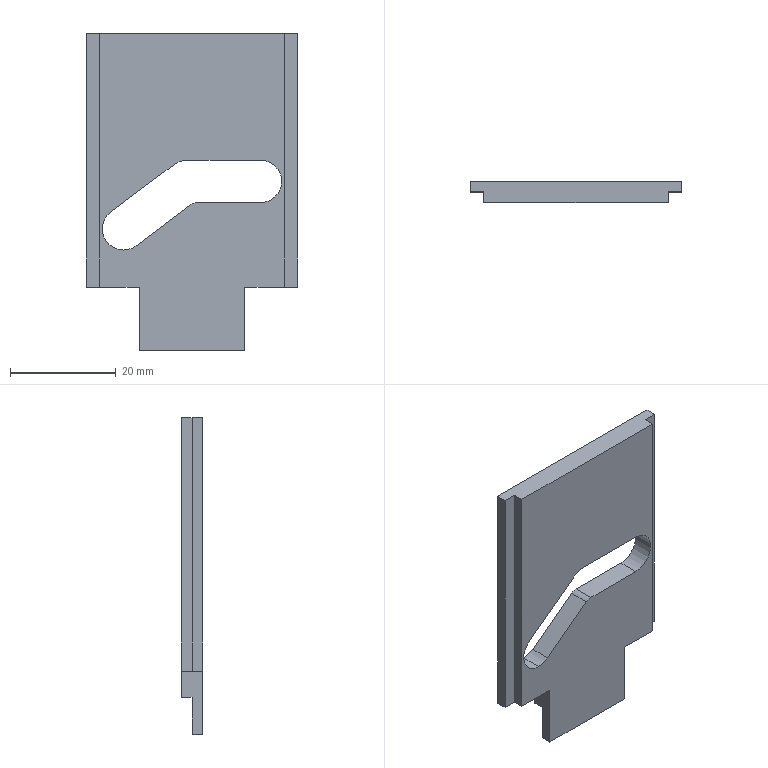Part | SolidWorks | features BaseBody 1 | 1 solid | 25 faces | box 40 x 4 x 60 mm | volume 6751 mm3 | plane 20 | cylinder 5 | commonest cylinder face diameters 8 x4 4 x1
STEP:
#1=CARTESIAN_POINT('',(-13.,4.,-17.));
#2=VERTEX_POINT('',#1);
#3=CARTESIAN_POINT('',(-10.6,4.,-16.2));
#4=VERTEX_POINT('',#3);
#5=CARTESIAN_POINT('',(-13.,4.,-13.));
#6=DIRECTION('',(0.,-1.,0.));
#7=DIRECTION('',(0.,0.,-1.));
#8=AXIS2_PLACEMENT_3D('',#5,#6,#7);
#9=CIRCLE('',#8,4.);
#10=EDGE_CURVE('',#2,#4,#9,.T.);
#11=ORIENTED_EDGE('',*,*,#10,.F.);
#12=CARTESIAN_POINT('',(-13.,0.,-17.));
#13=VERTEX_POINT('',#12);
#14=CARTESIAN_POINT('',(-13.,4.,-17.));
#15=DIRECTION('',(0.,-1.,0.));
#16=VECTOR('',#15,1000.);
#17=LINE('',#14,#16);
#18=EDGE_CURVE('',#2,#13,#17,.T.);
#19=ORIENTED_EDGE('',*,*,#18,.T.);
#20=CARTESIAN_POINT('',(-10.6,0.,-16.2));
#21=VERTEX_POINT('',#20);
#22=CARTESIAN_POINT('',(-13.,0.,-13.));
#23=DIRECTION('',(0.,1.,0.));
#24=DIRECTION('',(0.,0.,-1.));
#25=AXIS2_PLACEMENT_3D('',#22,#23,#24);
#26=CIRCLE('',#25,4.);
#27=EDGE_CURVE('',#21,#13,#26,.T.);
#28=ORIENTED_EDGE('',*,*,#27,.F.);
#29=CARTESIAN_POINT('',(-10.6,4.,-16.2));
#30=DIRECTION('',(0.,-1.,0.));
#31=VECTOR('',#30,1000.);
#32=LINE('',#29,#31);
#33=EDGE_CURVE('',#4,#21,#32,.T.);
#34=ORIENTED_EDGE('',*,*,#33,.F.);
#35=EDGE_LOOP('',(#11,#19,#28,#34));
#36=FACE_OUTER_BOUND('',#35,.T.);
#37=CARTESIAN_POINT('',(-13.,4.,-13.));
#38=DIRECTION('',(0.,-1.,0.));
#39=DIRECTION('',(0.,0.,-1.));
#40=AXIS2_PLACEMENT_3D('',#37,#38,#39);
#41=CYLINDRICAL_SURFACE('',#40,4.);
#42=ADVANCED_FACE('',(#36),#41,.F.);
#43=CARTESIAN_POINT('',(-15.4,4.,-9.8));
#44=VERTEX_POINT('',#43);
#45=CARTESIAN_POINT('',(-13.,4.,-13.));
#46=DIRECTION('',(0.,-1.,0.));
#47=DIRECTION('',(0.,0.,-1.));
#48=AXIS2_PLACEMENT_3D('',#45,#46,#47);
#49=CIRCLE('',#48,4.);
#50=EDGE_CURVE('',#44,#2,#49,.T.);
#51=ORIENTED_EDGE('',*,*,#50,.T.);
#52=ORIENTED_EDGE('',*,*,#10,.T.);
#53=CARTESIAN_POINT('',(-0.2,4.,-8.4));
#54=VERTEX_POINT('',#53);
#55=CARTESIAN_POINT('',(-10.6,4.,-16.2));
#56=DIRECTION('',(0.8,0.,0.6));
#57=VECTOR('',#56,1000.);
#58=LINE('',#55,#57);
#59=EDGE_CURVE('',#4,#54,#58,.T.);
#60=ORIENTED_EDGE('',*,*,#59,.T.);
#61=CARTESIAN_POINT('',(1.,4.,-8.));
#62=VERTEX_POINT('',#61);
#63=CARTESIAN_POINT('',(1.,4.,-10.));
#64=DIRECTION('',(0.,-1.,0.));
#65=DIRECTION('',(0.,0.,-1.));
#66=AXIS2_PLACEMENT_3D('',#63,#64,#65);
#67=CIRCLE('',#66,2.);
#68=EDGE_CURVE('',#62,#54,#67,.T.);
#69=ORIENTED_EDGE('',*,*,#68,.F.);
#70=CARTESIAN_POINT('',(13.,4.,-8.));
#71=VERTEX_POINT('',#70);
#72=CARTESIAN_POINT('',(0.,4.,-8.));
#73=DIRECTION('',(1.,0.,0.));
#74=VECTOR('',#73,1000.);
#75=LINE('',#72,#74);
#76=EDGE_CURVE('',#62,#71,#75,.T.);
#77=ORIENTED_EDGE('',*,*,#76,.T.);
#78=CARTESIAN_POINT('',(13.,4.,0.));
#79=VERTEX_POINT('',#78);
#80=CARTESIAN_POINT('',(13.,4.,-4.));
#81=DIRECTION('',(0.,-1.,0.));
#82=DIRECTION('',(0.,0.,-1.));
#83=AXIS2_PLACEMENT_3D('',#80,#81,#82);
#84=CIRCLE('',#83,4.);
#85=EDGE_CURVE('',#71,#79,#84,.T.);
#86=ORIENTED_EDGE('',*,*,#85,.T.);
#87=CARTESIAN_POINT('',(-1.,4.,0.));
#88=VERTEX_POINT('',#87);
#89=CARTESIAN_POINT('',(0.,4.,0.));
#90=DIRECTION('',(-1.,0.,0.));
#91=VECTOR('',#90,1000.);
#92=LINE('',#89,#91);
#93=EDGE_CURVE('',#79,#88,#92,.T.);
#94=ORIENTED_EDGE('',*,*,#93,.T.);
#95=CARTESIAN_POINT('',(-3.4,4.,-0.8));
#96=VERTEX_POINT('',#95);
#97=CARTESIAN_POINT('',(-1.,4.,-4.));
#98=DIRECTION('',(0.,-1.,0.));
#99=DIRECTION('',(0.,0.,-1.));
#100=AXIS2_PLACEMENT_3D('',#97,#98,#99);
#101=CIRCLE('',#100,4.);
#102=EDGE_CURVE('',#88,#96,#101,.T.);
#103=ORIENTED_EDGE('',*,*,#102,.T.);
#104=CARTESIAN_POINT('',(-3.4,4.,-0.8));
#105=DIRECTION('',(-0.8,0.,-0.6));
#106=VECTOR('',#105,1000.);
#107=LINE('',#104,#106);
#108=EDGE_CURVE('',#96,#44,#107,.T.);
#109=ORIENTED_EDGE('',*,*,#108,.T.);
#110=EDGE_LOOP('',(#51,#52,#60,#69,#77,#86,#94,#103,#109));
#111=FACE_BOUND('',#110,.T.);
#112=CARTESIAN_POINT('',(20.,4.,-24.));
#113=VERTEX_POINT('',#112);
#114=CARTESIAN_POINT('',(10.,4.,-24.));
#115=VERTEX_POINT('',#114);
#116=CARTESIAN_POINT('',(0.,4.,-24.));
#117=DIRECTION('',(-1.,0.,0.));
#118=VECTOR('',#117,1000.);
#119=LINE('',#116,#118);
#120=EDGE_CURVE('',#113,#115,#119,.T.);
#121=ORIENTED_EDGE('',*,*,#120,.T.);
#122=CARTESIAN_POINT('',(10.,4.,-29.));
#123=VERTEX_POINT('',#122);
#124=CARTESIAN_POINT('',(10.,4.,0.));
#125=DIRECTION('',(0.,0.,-1.));
#126=VECTOR('',#125,1000.);
#127=LINE('',#124,#126);
#128=EDGE_CURVE('',#115,#123,#127,.T.);
#129=ORIENTED_EDGE('',*,*,#128,.T.);
#130=CARTESIAN_POINT('',(-10.,4.,-29.));
#131=VERTEX_POINT('',#130);
#132=CARTESIAN_POINT('',(0.,4.,-29.));
#133=DIRECTION('',(-1.,0.,0.));
#134=VECTOR('',#133,1000.);
#135=LINE('',#132,#134);
#136=EDGE_CURVE('',#123,#131,#135,.T.);
#137=ORIENTED_EDGE('',*,*,#136,.T.);
#138=CARTESIAN_POINT('',(-10.,4.,-24.));
#139=VERTEX_POINT('',#138);
#140=CARTESIAN_POINT('',(-10.,4.,0.));
#141=DIRECTION('',(0.,0.,1.));
#142=VECTOR('',#141,1000.);
#143=LINE('',#140,#142);
#144=EDGE_CURVE('',#131,#139,#143,.T.);
#145=ORIENTED_EDGE('',*,*,#144,.T.);
#146=CARTESIAN_POINT('',(-20.,4.,-24.));
#147=VERTEX_POINT('',#146);
#148=CARTESIAN_POINT('',(0.,4.,-24.));
#149=DIRECTION('',(-1.,0.,0.));
#150=VECTOR('',#149,1000.);
#151=LINE('',#148,#150);
#152=EDGE_CURVE('',#139,#147,#151,.T.);
#153=ORIENTED_EDGE('',*,*,#152,.T.);
#154=CARTESIAN_POINT('',(-20.,4.,24.));
#155=VERTEX_POINT('',#154);
#156=CARTESIAN_POINT('',(-20.,4.,0.));
#157=DIRECTION('',(0.,0.,1.));
#158=VECTOR('',#157,1000.);
#159=LINE('',#156,#158);
#160=EDGE_CURVE('',#147,#155,#159,.T.);
#161=ORIENTED_EDGE('',*,*,#160,.T.);
#162=CARTESIAN_POINT('',(20.,4.,24.));
#163=VERTEX_POINT('',#162);
#164=CARTESIAN_POINT('',(0.,4.,24.));
#165=DIRECTION('',(1.,0.,0.));
#166=VECTOR('',#165,1000.);
#167=LINE('',#164,#166);
#168=EDGE_CURVE('',#155,#163,#167,.T.);
#169=ORIENTED_EDGE('',*,*,#168,.T.);
#170=CARTESIAN_POINT('',(20.,4.,0.));
#171=DIRECTION('',(0.,0.,-1.));
#172=VECTOR('',#171,1000.);
#173=LINE('',#170,#172);
#174=EDGE_CURVE('',#163,#113,#173,.T.);
#175=ORIENTED_EDGE('',*,*,#174,.T.);
#176=EDGE_LOOP('',(#121,#129,#137,#145,#153,#161,#169,#175));
#177=FACE_OUTER_BOUND('',#176,.T.);
#178=CARTESIAN_POINT('',(0.,4.,0.));
#179=DIRECTION('',(0.,1.,0.));
#180=DIRECTION('',(0.,0.,1.));
#181=AXIS2_PLACEMENT_3D('',#178,#179,#180);
#182=PLANE('',#181);
#183=ADVANCED_FACE('',(#111,#177),#182,.T.);
#184=ORIENTED_EDGE('',*,*,#18,.F.);
#185=ORIENTED_EDGE('',*,*,#50,.F.);
#186=CARTESIAN_POINT('',(-15.4,0.,-9.8));
#187=VERTEX_POINT('',#186);
#188=CARTESIAN_POINT('',(-15.4,4.,-9.8));
#189=DIRECTION('',(0.,1.,0.));
#190=VECTOR('',#189,1000.);
#191=LINE('',#188,#190);
#192=EDGE_CURVE('',#187,#44,#191,.T.);
#193=ORIENTED_EDGE('',*,*,#192,.F.);
#194=CARTESIAN_POINT('',(-13.,0.,-13.));
#195=DIRECTION('',(0.,1.,0.));
#196=DIRECTION('',(0.,0.,-1.));
#197=AXIS2_PLACEMENT_3D('',#194,#195,#196);
#198=CIRCLE('',#197,4.);
#199=EDGE_CURVE('',#13,#187,#198,.T.);
#200=ORIENTED_EDGE('',*,*,#199,.F.);
#201=EDGE_LOOP('',(#184,#185,#193,#200));
#202=FACE_OUTER_BOUND('',#201,.T.);
#203=CARTESIAN_POINT('',(-13.,4.,-13.));
#204=DIRECTION('',(0.,-1.,0.));
#205=DIRECTION('',(0.,0.,-1.));
#206=AXIS2_PLACEMENT_3D('',#203,#204,#205);
#207=CYLINDRICAL_SURFACE('',#206,4.);
#208=ADVANCED_FACE('',(#202),#207,.F.);
#209=ORIENTED_EDGE('',*,*,#192,.T.);
#210=ORIENTED_EDGE('',*,*,#108,.F.);
#211=CARTESIAN_POINT('',(-3.4,0.,-0.8));
#212=VERTEX_POINT('',#211);
#213=CARTESIAN_POINT('',(-3.4,4.,-0.8));
#214=DIRECTION('',(0.,1.,0.));
#215=VECTOR('',#214,1000.);
#216=LINE('',#213,#215);
#217=EDGE_CURVE('',#212,#96,#216,.T.);
#218=ORIENTED_EDGE('',*,*,#217,.F.);
#219=CARTESIAN_POINT('',(-0.84,0.,1.12));
#220=DIRECTION('',(0.8,0.,0.6));
#221=VECTOR('',#220,1000.);
#222=LINE('',#219,#221);
#223=EDGE_CURVE('',#187,#212,#222,.T.);
#224=ORIENTED_EDGE('',*,*,#223,.F.);
#225=EDGE_LOOP('',(#209,#210,#218,#224));
#226=FACE_OUTER_BOUND('',#225,.T.);
#227=CARTESIAN_POINT('',(-0.84,4.,1.12));
#228=DIRECTION('',(-0.6,0.,0.8));
#229=DIRECTION('',(0.8,0.,0.6));
#230=AXIS2_PLACEMENT_3D('',#227,#228,#229);
#231=PLANE('',#230);
#232=ADVANCED_FACE('',(#226),#231,.F.);
#233=ORIENTED_EDGE('',*,*,#217,.T.);
#234=ORIENTED_EDGE('',*,*,#102,.F.);
#235=CARTESIAN_POINT('',(-1.,0.,0.));
#236=VERTEX_POINT('',#235);
#237=CARTESIAN_POINT('',(-1.,4.,0.));
#238=DIRECTION('',(0.,1.,0.));
#239=VECTOR('',#238,1000.);
#240=LINE('',#237,#239);
#241=EDGE_CURVE('',#236,#88,#240,.T.);
#242=ORIENTED_EDGE('',*,*,#241,.F.);
#243=CARTESIAN_POINT('',(-1.,0.,-4.));
#244=DIRECTION('',(0.,1.,0.));
#245=DIRECTION('',(0.,0.,-1.));
#246=AXIS2_PLACEMENT_3D('',#243,#244,#245);
#247=CIRCLE('',#246,4.);
#248=EDGE_CURVE('',#212,#236,#247,.T.);
#249=ORIENTED_EDGE('',*,*,#248,.F.);
#250=EDGE_LOOP('',(#233,#234,#242,#249));
#251=FACE_OUTER_BOUND('',#250,.T.);
#252=CARTESIAN_POINT('',(-1.,4.,-4.));
#253=DIRECTION('',(0.,-1.,0.));
#254=DIRECTION('',(0.,0.,-1.));
#255=AXIS2_PLACEMENT_3D('',#252,#253,#254);
#256=CYLINDRICAL_SURFACE('',#255,4.);
#257=ADVANCED_FACE('',(#251),#256,.F.);
#258=ORIENTED_EDGE('',*,*,#93,.F.);
#259=CARTESIAN_POINT('',(13.,0.,0.));
#260=VERTEX_POINT('',#259);
#261=CARTESIAN_POINT('',(13.,4.,0.));
#262=DIRECTION('',(0.,-1.,0.));
#263=VECTOR('',#262,1000.);
#264=LINE('',#261,#263);
#265=EDGE_CURVE('',#79,#260,#264,.T.);
#266=ORIENTED_EDGE('',*,*,#265,.T.);
#267=CARTESIAN_POINT('',(0.,0.,0.));
#268=DIRECTION('',(-1.,0.,0.));
#269=VECTOR('',#268,1000.);
#270=LINE('',#267,#269);
#271=EDGE_CURVE('',#260,#236,#270,.T.);
#272=ORIENTED_EDGE('',*,*,#271,.T.);
#273=ORIENTED_EDGE('',*,*,#241,.T.);
#274=EDGE_LOOP('',(#258,#266,#272,#273));
#275=FACE_OUTER_BOUND('',#274,.T.);
#276=CARTESIAN_POINT('',(0.,4.,0.));
#277=DIRECTION('',(0.,0.,-1.));
#278=DIRECTION('',(-1.,0.,0.));
#279=AXIS2_PLACEMENT_3D('',#276,#277,#278);
#280=PLANE('',#279);
#281=ADVANCED_FACE('',(#275),#280,.T.);
#282=ORIENTED_EDGE('',*,*,#265,.F.);
#283=ORIENTED_EDGE('',*,*,#85,.F.);
#284=CARTESIAN_POINT('',(13.,0.,-8.));
#285=VERTEX_POINT('',#284);
#286=CARTESIAN_POINT('',(13.,4.,-8.));
#287=DIRECTION('',(0.,1.,0.));
#288=VECTOR('',#287,1000.);
#289=LINE('',#286,#288);
#290=EDGE_CURVE('',#285,#71,#289,.T.);
#291=ORIENTED_EDGE('',*,*,#290,.F.);
#292=CARTESIAN_POINT('',(13.,0.,-4.));
#293=DIRECTION('',(0.,1.,0.));
#294=DIRECTION('',(0.,0.,-1.));
#295=AXIS2_PLACEMENT_3D('',#292,#293,#294);
#296=CIRCLE('',#295,4.);
#297=EDGE_CURVE('',#260,#285,#296,.T.);
#298=ORIENTED_EDGE('',*,*,#297,.F.);
#299=EDGE_LOOP('',(#282,#283,#291,#298));
#300=FACE_OUTER_BOUND('',#299,.T.);
#301=CARTESIAN_POINT('',(13.,4.,-4.));
#302=DIRECTION('',(0.,-1.,0.));
#303=DIRECTION('',(0.,0.,-1.));
#304=AXIS2_PLACEMENT_3D('',#301,#302,#303);
#305=CYLINDRICAL_SURFACE('',#304,4.);
#306=ADVANCED_FACE('',(#300),#305,.F.);
#307=ORIENTED_EDGE('',*,*,#290,.T.);
#308=ORIENTED_EDGE('',*,*,#76,.F.);
#309=CARTESIAN_POINT('',(1.,0.,-8.));
#310=VERTEX_POINT('',#309);
#311=CARTESIAN_POINT('',(1.,4.,-8.));
#312=DIRECTION('',(0.,1.,0.));
#313=VECTOR('',#312,1000.);
#314=LINE('',#311,#313);
#315=EDGE_CURVE('',#310,#62,#314,.T.);
#316=ORIENTED_EDGE('',*,*,#315,.F.);
#317=CARTESIAN_POINT('',(0.,0.,-8.));
#318=DIRECTION('',(-1.,0.,0.));
#319=VECTOR('',#318,1000.);
#320=LINE('',#317,#319);
#321=EDGE_CURVE('',#285,#310,#320,.T.);
#322=ORIENTED_EDGE('',*,*,#321,.F.);
#323=EDGE_LOOP('',(#307,#308,#316,#322));
#324=FACE_OUTER_BOUND('',#323,.T.);
#325=CARTESIAN_POINT('',(0.,4.,-8.));
#326=DIRECTION('',(0.,0.,-1.));
#327=DIRECTION('',(-1.,0.,0.));
#328=AXIS2_PLACEMENT_3D('',#325,#326,#327);
#329=PLANE('',#328);
#330=ADVANCED_FACE('',(#324),#329,.F.);
#331=ORIENTED_EDGE('',*,*,#59,.F.);
#332=ORIENTED_EDGE('',*,*,#33,.T.);
#333=CARTESIAN_POINT('',(-0.2,0.,-8.4));
#334=VERTEX_POINT('',#333);
#335=CARTESIAN_POINT('',(3.96,0.,-5.28));
#336=DIRECTION('',(0.8,0.,0.6));
#337=VECTOR('',#336,1000.);
#338=LINE('',#335,#337);
#339=EDGE_CURVE('',#21,#334,#338,.T.);
#340=ORIENTED_EDGE('',*,*,#339,.T.);
#341=CARTESIAN_POINT('',(-0.2,4.,-8.4));
#342=DIRECTION('',(0.,1.,0.));
#343=VECTOR('',#342,1000.);
#344=LINE('',#341,#343);
#345=EDGE_CURVE('',#334,#54,#344,.T.);
#346=ORIENTED_EDGE('',*,*,#345,.T.);
#347=EDGE_LOOP('',(#331,#332,#340,#346));
#348=FACE_OUTER_BOUND('',#347,.T.);
#349=CARTESIAN_POINT('',(3.96,4.,-5.28));
#350=DIRECTION('',(-0.6,0.,0.8));
#351=DIRECTION('',(0.8,0.,0.6));
#352=AXIS2_PLACEMENT_3D('',#349,#350,#351);
#353=PLANE('',#352);
#354=ADVANCED_FACE('',(#348),#353,.T.);
#355=CARTESIAN_POINT('',(10.,0.,-36.));
#356=VERTEX_POINT('',#355);
#357=CARTESIAN_POINT('',(10.,2.,-36.));
#358=VERTEX_POINT('',#357);
#359=CARTESIAN_POINT('',(10.,4.,-36.));
#360=DIRECTION('',(0.,1.,0.));
#361=VECTOR('',#360,1000.);
#362=LINE('',#359,#361);
#363=EDGE_CURVE('',#356,#358,#362,.T.);
#364=ORIENTED_EDGE('',*,*,#363,.T.);
#365=CARTESIAN_POINT('',(10.,2.,-29.));
#366=VERTEX_POINT('',#365);
#367=CARTESIAN_POINT('',(10.,2.,0.));
#368=DIRECTION('',(0.,0.,1.));
#369=VECTOR('',#368,1000.);
#370=LINE('',#367,#369);
#371=EDGE_CURVE('',#358,#366,#370,.T.);
#372=ORIENTED_EDGE('',*,*,#371,.T.);
#373=CARTESIAN_POINT('',(10.,4.,-29.));
#374=DIRECTION('',(0.,1.,0.));
#375=VECTOR('',#374,1000.);
#376=LINE('',#373,#375);
#377=EDGE_CURVE('',#366,#123,#376,.T.);
#378=ORIENTED_EDGE('',*,*,#377,.T.);
#379=ORIENTED_EDGE('',*,*,#128,.F.);
#380=CARTESIAN_POINT('',(10.,0.,-24.));
#381=VERTEX_POINT('',#380);
#382=CARTESIAN_POINT('',(10.,4.,-24.));
#383=DIRECTION('',(0.,-1.,0.));
#384=VECTOR('',#383,1000.);
#385=LINE('',#382,#384);
#386=EDGE_CURVE('',#115,#381,#385,.T.);
#387=ORIENTED_EDGE('',*,*,#386,.T.);
#388=CARTESIAN_POINT('',(10.,0.,0.));
#389=DIRECTION('',(0.,0.,-1.));
#390=VECTOR('',#389,1000.);
#391=LINE('',#388,#390);
#392=EDGE_CURVE('',#381,#356,#391,.T.);
#393=ORIENTED_EDGE('',*,*,#392,.T.);
#394=EDGE_LOOP('',(#364,#372,#378,#379,#387,#393));
#395=FACE_OUTER_BOUND('',#394,.T.);
#396=CARTESIAN_POINT('',(10.,4.,0.));
#397=DIRECTION('',(1.,0.,0.));
#398=DIRECTION('',(0.,0.,-1.));
#399=AXIS2_PLACEMENT_3D('',#396,#397,#398);
#400=PLANE('',#399);
#401=ADVANCED_FACE('',(#395),#400,.T.);
#402=CARTESIAN_POINT('',(20.,2.,-24.));
#403=VERTEX_POINT('',#402);
#404=CARTESIAN_POINT('',(20.,4.,-24.));
#405=DIRECTION('',(0.,-1.,0.));
#406=VECTOR('',#405,1000.);
#407=LINE('',#404,#406);
#408=EDGE_CURVE('',#113,#403,#407,.T.);
#409=ORIENTED_EDGE('',*,*,#408,.T.);
#410=CARTESIAN_POINT('',(17.5,2.,-24.));
#411=VERTEX_POINT('',#410);
#412=CARTESIAN_POINT('',(0.,2.,-24.));
#413=DIRECTION('',(-1.,0.,0.));
#414=VECTOR('',#413,1000.);
#415=LINE('',#412,#414);
#416=EDGE_CURVE('',#403,#411,#415,.T.);
#417=ORIENTED_EDGE('',*,*,#416,.T.);
#418=CARTESIAN_POINT('',(17.5,0.,-24.));
#419=VERTEX_POINT('',#418);
#420=CARTESIAN_POINT('',(17.5,4.,-24.));
#421=DIRECTION('',(0.,-1.,0.));
#422=VECTOR('',#421,1000.);
#423=LINE('',#420,#422);
#424=EDGE_CURVE('',#411,#419,#423,.T.);
#425=ORIENTED_EDGE('',*,*,#424,.T.);
#426=CARTESIAN_POINT('',(0.,0.,-24.));
#427=DIRECTION('',(-1.,0.,0.));
#428=VECTOR('',#427,1000.);
#429=LINE('',#426,#428);
#430=EDGE_CURVE('',#419,#381,#429,.T.);
#431=ORIENTED_EDGE('',*,*,#430,.T.);
#432=ORIENTED_EDGE('',*,*,#386,.F.);
#433=ORIENTED_EDGE('',*,*,#120,.F.);
#434=EDGE_LOOP('',(#409,#417,#425,#431,#432,#433));
#435=FACE_OUTER_BOUND('',#434,.T.);
#436=CARTESIAN_POINT('',(0.,4.,-24.));
#437=DIRECTION('',(0.,0.,-1.));
#438=DIRECTION('',(-1.,0.,0.));
#439=AXIS2_PLACEMENT_3D('',#436,#437,#438);
#440=PLANE('',#439);
#441=ADVANCED_FACE('',(#435),#440,.T.);
#442=CARTESIAN_POINT('',(20.,2.,24.));
#443=VERTEX_POINT('',#442);
#444=CARTESIAN_POINT('',(20.,2.,0.));
#445=DIRECTION('',(0.,0.,1.));
#446=VECTOR('',#445,1000.);
#447=LINE('',#444,#446);
#448=EDGE_CURVE('',#403,#443,#447,.T.);
#449=ORIENTED_EDGE('',*,*,#448,.F.);
#450=ORIENTED_EDGE('',*,*,#408,.F.);
#451=ORIENTED_EDGE('',*,*,#174,.F.);
#452=CARTESIAN_POINT('',(20.,4.,24.));
#453=DIRECTION('',(0.,1.,0.));
#454=VECTOR('',#453,1000.);
#455=LINE('',#452,#454);
#456=EDGE_CURVE('',#443,#163,#455,.T.);
#457=ORIENTED_EDGE('',*,*,#456,.F.);
#458=EDGE_LOOP('',(#449,#450,#451,#457));
#459=FACE_OUTER_BOUND('',#458,.T.);
#460=CARTESIAN_POINT('',(20.,4.,0.));
#461=DIRECTION('',(-1.,0.,0.));
#462=DIRECTION('',(0.,0.,1.));
#463=AXIS2_PLACEMENT_3D('',#460,#461,#462);
#464=PLANE('',#463);
#465=ADVANCED_FACE('',(#459),#464,.F.);
#466=CARTESIAN_POINT('',(-17.5,0.,24.));
#467=VERTEX_POINT('',#466);
#468=CARTESIAN_POINT('',(-17.5,2.,24.));
#469=VERTEX_POINT('',#468);
#470=CARTESIAN_POINT('',(-17.5,4.,24.));
#471=DIRECTION('',(0.,1.,0.));
#472=VECTOR('',#471,1000.);
#473=LINE('',#470,#472);
#474=EDGE_CURVE('',#467,#469,#473,.T.);
#475=ORIENTED_EDGE('',*,*,#474,.F.);
#476=CARTESIAN_POINT('',(17.5,0.,24.));
#477=VERTEX_POINT('',#476);
#478=CARTESIAN_POINT('',(0.,0.,24.));
#479=DIRECTION('',(-1.,0.,0.));
#480=VECTOR('',#479,1000.);
#481=LINE('',#478,#480);
#482=EDGE_CURVE('',#477,#467,#481,.T.);
#483=ORIENTED_EDGE('',*,*,#482,.F.);
#484=CARTESIAN_POINT('',(17.5,2.,24.));
#485=VERTEX_POINT('',#484);
#486=CARTESIAN_POINT('',(17.5,4.,24.));
#487=DIRECTION('',(0.,-1.,0.));
#488=VECTOR('',#487,1000.);
#489=LINE('',#486,#488);
#490=EDGE_CURVE('',#485,#477,#489,.T.);
#491=ORIENTED_EDGE('',*,*,#490,.F.);
#492=CARTESIAN_POINT('',(0.,2.,24.));
#493=DIRECTION('',(-1.,0.,0.));
#494=VECTOR('',#493,1000.);
#495=LINE('',#492,#494);
#496=EDGE_CURVE('',#443,#485,#495,.T.);
#497=ORIENTED_EDGE('',*,*,#496,.F.);
#498=ORIENTED_EDGE('',*,*,#456,.T.);
#499=ORIENTED_EDGE('',*,*,#168,.F.);
#500=CARTESIAN_POINT('',(-20.,2.,24.));
#501=VERTEX_POINT('',#500);
#502=CARTESIAN_POINT('',(-20.,4.,24.));
#503=DIRECTION('',(0.,1.,0.));
#504=VECTOR('',#503,1000.);
#505=LINE('',#502,#504);
#506=EDGE_CURVE('',#501,#155,#505,.T.);
#507=ORIENTED_EDGE('',*,*,#506,.F.);
#508=CARTESIAN_POINT('',(0.,2.,24.));
#509=DIRECTION('',(-1.,0.,0.));
#510=VECTOR('',#509,1000.);
#511=LINE('',#508,#510);
#512=EDGE_CURVE('',#469,#501,#511,.T.);
#513=ORIENTED_EDGE('',*,*,#512,.F.);
#514=EDGE_LOOP('',(#475,#483,#491,#497,#498,#499,#507,#513));
#515=FACE_OUTER_BOUND('',#514,.T.);
#516=CARTESIAN_POINT('',(0.,4.,24.));
#517=DIRECTION('',(0.,0.,-1.));
#518=DIRECTION('',(-1.,0.,0.));
#519=AXIS2_PLACEMENT_3D('',#516,#517,#518);
#520=PLANE('',#519);
#521=ADVANCED_FACE('',(#515),#520,.F.);
#522=ORIENTED_EDGE('',*,*,#506,.T.);
#523=ORIENTED_EDGE('',*,*,#160,.F.);
#524=CARTESIAN_POINT('',(-20.,2.,-24.));
#525=VERTEX_POINT('',#524);
#526=CARTESIAN_POINT('',(-20.,4.,-24.));
#527=DIRECTION('',(0.,-1.,0.));
#528=VECTOR('',#527,1000.);
#529=LINE('',#526,#528);
#530=EDGE_CURVE('',#147,#525,#529,.T.);
#531=ORIENTED_EDGE('',*,*,#530,.T.);
#532=CARTESIAN_POINT('',(-20.,2.,0.));
#533=DIRECTION('',(0.,0.,1.));
#534=VECTOR('',#533,1000.);
#535=LINE('',#532,#534);
#536=EDGE_CURVE('',#525,#501,#535,.T.);
#537=ORIENTED_EDGE('',*,*,#536,.T.);
#538=EDGE_LOOP('',(#522,#523,#531,#537));
#539=FACE_OUTER_BOUND('',#538,.T.);
#540=CARTESIAN_POINT('',(-20.,4.,0.));
#541=DIRECTION('',(-1.,0.,0.));
#542=DIRECTION('',(0.,0.,1.));
#543=AXIS2_PLACEMENT_3D('',#540,#541,#542);
#544=PLANE('',#543);
#545=ADVANCED_FACE('',(#539),#544,.T.);
#546=CARTESIAN_POINT('',(-10.,0.,-24.));
#547=VERTEX_POINT('',#546);
#548=CARTESIAN_POINT('',(-10.,4.,-24.));
#549=DIRECTION('',(0.,-1.,0.));
#550=VECTOR('',#549,1000.);
#551=LINE('',#548,#550);
#552=EDGE_CURVE('',#139,#547,#551,.T.);
#553=ORIENTED_EDGE('',*,*,#552,.T.);
#554=CARTESIAN_POINT('',(-17.5,0.,-24.));
#555=VERTEX_POINT('',#554);
#556=CARTESIAN_POINT('',(0.,0.,-24.));
#557=DIRECTION('',(-1.,0.,0.));
#558=VECTOR('',#557,1000.);
#559=LINE('',#556,#558);
#560=EDGE_CURVE('',#547,#555,#559,.T.);
#561=ORIENTED_EDGE('',*,*,#560,.T.);
#562=CARTESIAN_POINT('',(-17.5,2.,-24.));
#563=VERTEX_POINT('',#562);
#564=CARTESIAN_POINT('',(-17.5,4.,-24.));
#565=DIRECTION('',(0.,1.,0.));
#566=VECTOR('',#565,1000.);
#567=LINE('',#564,#566);
#568=EDGE_CURVE('',#555,#563,#567,.T.);
#569=ORIENTED_EDGE('',*,*,#568,.T.);
#570=CARTESIAN_POINT('',(0.,2.,-24.));
#571=DIRECTION('',(-1.,0.,0.));
#572=VECTOR('',#571,1000.);
#573=LINE('',#570,#572);
#574=EDGE_CURVE('',#563,#525,#573,.T.);
#575=ORIENTED_EDGE('',*,*,#574,.T.);
#576=ORIENTED_EDGE('',*,*,#530,.F.);
#577=ORIENTED_EDGE('',*,*,#152,.F.);
#578=EDGE_LOOP('',(#553,#561,#569,#575,#576,#577));
#579=FACE_OUTER_BOUND('',#578,.T.);
#580=CARTESIAN_POINT('',(0.,4.,-24.));
#581=DIRECTION('',(0.,0.,-1.));
#582=DIRECTION('',(-1.,0.,0.));
#583=AXIS2_PLACEMENT_3D('',#580,#581,#582);
#584=PLANE('',#583);
#585=ADVANCED_FACE('',(#579),#584,.T.);
#586=CARTESIAN_POINT('',(-10.,2.,-29.));
#587=VERTEX_POINT('',#586);
#588=CARTESIAN_POINT('',(-10.,4.,-29.));
#589=DIRECTION('',(0.,1.,0.));
#590=VECTOR('',#589,1000.);
#591=LINE('',#588,#590);
#592=EDGE_CURVE('',#587,#131,#591,.T.);
#593=ORIENTED_EDGE('',*,*,#592,.F.);
#594=CARTESIAN_POINT('',(-10.,2.,-36.));
#595=VERTEX_POINT('',#594);
#596=CARTESIAN_POINT('',(-10.,2.,0.));
#597=DIRECTION('',(0.,0.,1.));
#598=VECTOR('',#597,1000.);
#599=LINE('',#596,#598);
#600=EDGE_CURVE('',#595,#587,#599,.T.);
#601=ORIENTED_EDGE('',*,*,#600,.F.);
#602=CARTESIAN_POINT('',(-10.,0.,-36.));
#603=VERTEX_POINT('',#602);
#604=CARTESIAN_POINT('',(-10.,4.,-36.));
#605=DIRECTION('',(0.,1.,0.));
#606=VECTOR('',#605,1000.);
#607=LINE('',#604,#606);
#608=EDGE_CURVE('',#603,#595,#607,.T.);
#609=ORIENTED_EDGE('',*,*,#608,.F.);
#610=CARTESIAN_POINT('',(-10.,0.,0.));
#611=DIRECTION('',(0.,0.,-1.));
#612=VECTOR('',#611,1000.);
#613=LINE('',#610,#612);
#614=EDGE_CURVE('',#547,#603,#613,.T.);
#615=ORIENTED_EDGE('',*,*,#614,.F.);
#616=ORIENTED_EDGE('',*,*,#552,.F.);
#617=ORIENTED_EDGE('',*,*,#144,.F.);
#618=EDGE_LOOP('',(#593,#601,#609,#615,#616,#617));
#619=FACE_OUTER_BOUND('',#618,.T.);
#620=CARTESIAN_POINT('',(-10.,4.,0.));
#621=DIRECTION('',(1.,0.,0.));
#622=DIRECTION('',(0.,0.,-1.));
#623=AXIS2_PLACEMENT_3D('',#620,#621,#622);
#624=PLANE('',#623);
#625=ADVANCED_FACE('',(#619),#624,.F.);
#626=ORIENTED_EDGE('',*,*,#377,.F.);
#627=CARTESIAN_POINT('',(-10.,2.,-29.));
#628=DIRECTION('',(1.,0.,0.));
#629=VECTOR('',#628,1000.);
#630=LINE('',#627,#629);
#631=EDGE_CURVE('',#587,#366,#630,.T.);
#632=ORIENTED_EDGE('',*,*,#631,.F.);
#633=ORIENTED_EDGE('',*,*,#592,.T.);
#634=ORIENTED_EDGE('',*,*,#136,.F.);
#635=EDGE_LOOP('',(#626,#632,#633,#634));
#636=FACE_OUTER_BOUND('',#635,.T.);
#637=CARTESIAN_POINT('',(-10.,2.,-29.));
#638=DIRECTION('',(0.,0.,1.));
#639=DIRECTION('',(1.,0.,0.));
#640=AXIS2_PLACEMENT_3D('',#637,#638,#639);
#641=PLANE('',#640);
#642=ADVANCED_FACE('',(#636),#641,.F.);
#643=ORIENTED_EDGE('',*,*,#27,.T.);
#644=ORIENTED_EDGE('',*,*,#199,.T.);
#645=ORIENTED_EDGE('',*,*,#223,.T.);
#646=ORIENTED_EDGE('',*,*,#248,.T.);
#647=ORIENTED_EDGE('',*,*,#271,.F.);
#648=ORIENTED_EDGE('',*,*,#297,.T.);
#649=ORIENTED_EDGE('',*,*,#321,.T.);
#650=CARTESIAN_POINT('',(1.,0.,-10.));
#651=DIRECTION('',(0.,1.,0.));
#652=DIRECTION('',(0.,0.,-1.));
#653=AXIS2_PLACEMENT_3D('',#650,#651,#652);
#654=CIRCLE('',#653,2.);
#655=EDGE_CURVE('',#334,#310,#654,.T.);
#656=ORIENTED_EDGE('',*,*,#655,.F.);
#657=ORIENTED_EDGE('',*,*,#339,.F.);
#658=EDGE_LOOP('',(#643,#644,#645,#646,#647,#648,#649,#656,#657));
#659=FACE_BOUND('',#658,.T.);
#660=CARTESIAN_POINT('',(-17.5,0.,0.));
#661=DIRECTION('',(0.,0.,1.));
#662=VECTOR('',#661,1000.);
#663=LINE('',#660,#662);
#664=EDGE_CURVE('',#555,#467,#663,.T.);
#665=ORIENTED_EDGE('',*,*,#664,.F.);
#666=ORIENTED_EDGE('',*,*,#560,.F.);
#667=ORIENTED_EDGE('',*,*,#614,.T.);
#668=CARTESIAN_POINT('',(0.,0.,-36.));
#669=DIRECTION('',(-1.,0.,0.));
#670=VECTOR('',#669,1000.);
#671=LINE('',#668,#670);
#672=EDGE_CURVE('',#356,#603,#671,.T.);
#673=ORIENTED_EDGE('',*,*,#672,.F.);
#674=ORIENTED_EDGE('',*,*,#392,.F.);
#675=ORIENTED_EDGE('',*,*,#430,.F.);
#676=CARTESIAN_POINT('',(17.5,0.,0.));
#677=DIRECTION('',(0.,0.,-1.));
#678=VECTOR('',#677,1000.);
#679=LINE('',#676,#678);
#680=EDGE_CURVE('',#477,#419,#679,.T.);
#681=ORIENTED_EDGE('',*,*,#680,.F.);
#682=ORIENTED_EDGE('',*,*,#482,.T.);
#683=EDGE_LOOP('',(#665,#666,#667,#673,#674,#675,#681,#682));
#684=FACE_OUTER_BOUND('',#683,.T.);
#685=CARTESIAN_POINT('',(0.,0.,0.));
#686=DIRECTION('',(0.,1.,0.));
#687=DIRECTION('',(0.,0.,1.));
#688=AXIS2_PLACEMENT_3D('',#685,#686,#687);
#689=PLANE('',#688);
#690=ADVANCED_FACE('',(#659,#684),#689,.F.);
#691=ORIENTED_EDGE('',*,*,#68,.T.);
#692=ORIENTED_EDGE('',*,*,#345,.F.);
#693=ORIENTED_EDGE('',*,*,#655,.T.);
#694=ORIENTED_EDGE('',*,*,#315,.T.);
#695=EDGE_LOOP('',(#691,#692,#693,#694));
#696=FACE_OUTER_BOUND('',#695,.T.);
#697=CARTESIAN_POINT('',(1.,4.,-10.));
#698=DIRECTION('',(0.,-1.,0.));
#699=DIRECTION('',(0.,0.,-1.));
#700=AXIS2_PLACEMENT_3D('',#697,#698,#699);
#701=CYLINDRICAL_SURFACE('',#700,2.);
#702=ADVANCED_FACE('',(#696),#701,.T.);
#703=ORIENTED_EDGE('',*,*,#371,.F.);
#704=CARTESIAN_POINT('',(0.,2.,-36.));
#705=DIRECTION('',(-1.,0.,0.));
#706=VECTOR('',#705,1000.);
#707=LINE('',#704,#706);
#708=EDGE_CURVE('',#358,#595,#707,.T.);
#709=ORIENTED_EDGE('',*,*,#708,.T.);
#710=ORIENTED_EDGE('',*,*,#600,.T.);
#711=ORIENTED_EDGE('',*,*,#631,.T.);
#712=EDGE_LOOP('',(#703,#709,#710,#711));
#713=FACE_OUTER_BOUND('',#712,.T.);
#714=CARTESIAN_POINT('',(0.,2.,0.));
#715=DIRECTION('',(0.,1.,0.));
#716=DIRECTION('',(0.,0.,1.));
#717=AXIS2_PLACEMENT_3D('',#714,#715,#716);
#718=PLANE('',#717);
#719=ADVANCED_FACE('',(#713),#718,.T.);
#720=ORIENTED_EDGE('',*,*,#363,.F.);
#721=ORIENTED_EDGE('',*,*,#672,.T.);
#722=ORIENTED_EDGE('',*,*,#608,.T.);
#723=ORIENTED_EDGE('',*,*,#708,.F.);
#724=EDGE_LOOP('',(#720,#721,#722,#723));
#725=FACE_OUTER_BOUND('',#724,.T.);
#726=CARTESIAN_POINT('',(0.,4.,-36.));
#727=DIRECTION('',(0.,0.,-1.));
#728=DIRECTION('',(-1.,0.,0.));
#729=AXIS2_PLACEMENT_3D('',#726,#727,#728);
#730=PLANE('',#729);
#731=ADVANCED_FACE('',(#725),#730,.T.);
#732=ORIENTED_EDGE('',*,*,#496,.T.);
#733=CARTESIAN_POINT('',(17.5,2.,0.));
#734=DIRECTION('',(0.,0.,1.));
#735=VECTOR('',#734,1000.);
#736=LINE('',#733,#735);
#737=EDGE_CURVE('',#411,#485,#736,.T.);
#738=ORIENTED_EDGE('',*,*,#737,.F.);
#739=ORIENTED_EDGE('',*,*,#416,.F.);
#740=ORIENTED_EDGE('',*,*,#448,.T.);
#741=EDGE_LOOP('',(#732,#738,#739,#740));
#742=FACE_OUTER_BOUND('',#741,.T.);
#743=CARTESIAN_POINT('',(0.,2.,0.));
#744=DIRECTION('',(0.,1.,0.));
#745=DIRECTION('',(0.,0.,1.));
#746=AXIS2_PLACEMENT_3D('',#743,#744,#745);
#747=PLANE('',#746);
#748=ADVANCED_FACE('',(#742),#747,.F.);
#749=ORIENTED_EDGE('',*,*,#424,.F.);
#750=ORIENTED_EDGE('',*,*,#737,.T.);
#751=ORIENTED_EDGE('',*,*,#490,.T.);
#752=ORIENTED_EDGE('',*,*,#680,.T.);
#753=EDGE_LOOP('',(#749,#750,#751,#752));
#754=FACE_OUTER_BOUND('',#753,.T.);
#755=CARTESIAN_POINT('',(17.5,2.,24.));
#756=DIRECTION('',(-1.,0.,0.));
#757=DIRECTION('',(0.,0.,1.));
#758=AXIS2_PLACEMENT_3D('',#755,#756,#757);
#759=PLANE('',#758);
#760=ADVANCED_FACE('',(#754),#759,.F.);
#761=CARTESIAN_POINT('',(-17.5,2.,0.));
#762=DIRECTION('',(0.,0.,1.));
#763=VECTOR('',#762,1000.);
#764=LINE('',#761,#763);
#765=EDGE_CURVE('',#563,#469,#764,.T.);
#766=ORIENTED_EDGE('',*,*,#765,.T.);
#767=ORIENTED_EDGE('',*,*,#512,.T.);
#768=ORIENTED_EDGE('',*,*,#536,.F.);
#769=ORIENTED_EDGE('',*,*,#574,.F.);
#770=EDGE_LOOP('',(#766,#767,#768,#769));
#771=FACE_OUTER_BOUND('',#770,.T.);
#772=CARTESIAN_POINT('',(0.,2.,0.));
#773=DIRECTION('',(0.,-1.,0.));
#774=DIRECTION('',(0.,0.,-1.));
#775=AXIS2_PLACEMENT_3D('',#772,#773,#774);
#776=PLANE('',#775);
#777=ADVANCED_FACE('',(#771),#776,.T.);
#778=ORIENTED_EDGE('',*,*,#474,.T.);
#779=ORIENTED_EDGE('',*,*,#765,.F.);
#780=ORIENTED_EDGE('',*,*,#568,.F.);
#781=ORIENTED_EDGE('',*,*,#664,.T.);
#782=EDGE_LOOP('',(#778,#779,#780,#781));
#783=FACE_OUTER_BOUND('',#782,.T.);
#784=CARTESIAN_POINT('',(-17.5,2.,24.));
#785=DIRECTION('',(1.,0.,0.));
#786=DIRECTION('',(0.,0.,-1.));
#787=AXIS2_PLACEMENT_3D('',#784,#785,#786);
#788=PLANE('',#787);
#789=ADVANCED_FACE('',(#783),#788,.F.);
#790=CLOSED_SHELL('',(#42,#183,#208,#232,#257,#281,#306,#330,#354,#401,#441,#465,#521,#545,#585,#625,#642,#690,#702,#719,#731,#748,#760,#777,#789));
#791=MANIFOLD_SOLID_BREP('',#790);
#792=CARTESIAN_POINT('',(0.,0.,0.));
#793=DIRECTION('',(0.,0.,1.));
#794=DIRECTION('',(1.,0.,0.));
#795=AXIS2_PLACEMENT_3D('',#792,#793,#794);
#796=(LENGTH_UNIT()NAMED_UNIT(*)SI_UNIT(.MILLI.,.METRE.));
#797=UNCERTAINTY_MEASURE_WITH_UNIT(LENGTH_MEASURE(0.00001),#796,'','');
#798=(NAMED_UNIT(*)PLANE_ANGLE_UNIT()SI_UNIT($,.RADIAN.));
#799=(NAMED_UNIT(*)SI_UNIT($,.STERADIAN.)SOLID_ANGLE_UNIT());
#800=(GEOMETRIC_REPRESENTATION_CONTEXT(3)GLOBAL_UNCERTAINTY_ASSIGNED_CONTEXT((#797))GLOBAL_UNIT_ASSIGNED_CONTEXT((#796,#798,#799))REPRESENTATION_CONTEXT('',''));
#801=ADVANCED_BREP_SHAPE_REPRESENTATION('',(#791,#795),#800);